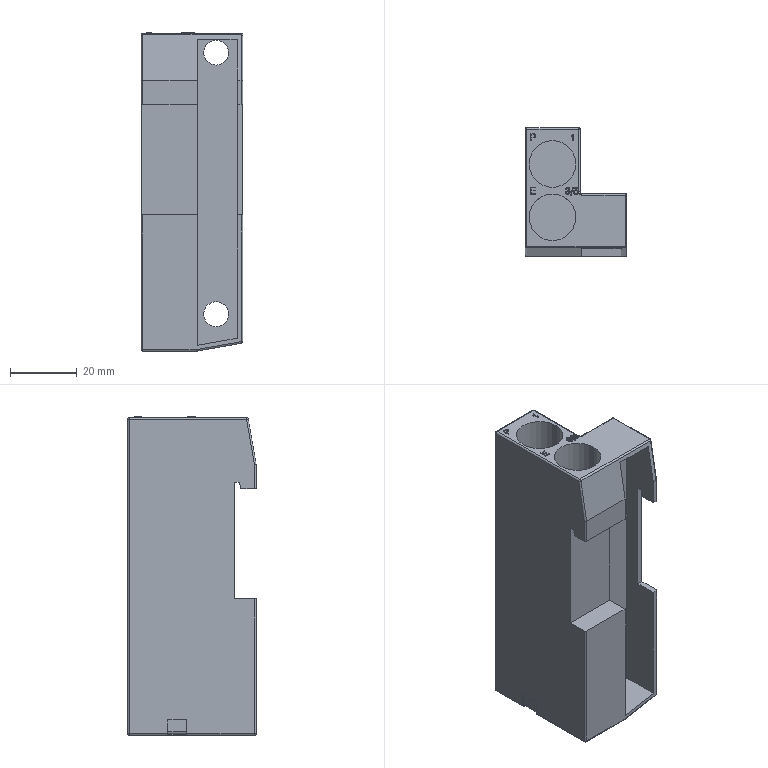Part | STEP file | SS5V1-16S3AD-08B-N1_CAD Side End Plate | 1 solid | 174 faces | box 30.5 x 38.5 x 95.55 mm | volume 62940 mm3 | plane 91 | cylinder 39 | spline 30 | sphere 12 | torus 2 | commonest cylinder face diameters 1 x25 2.5 x4 7.5 x4 14 x4 0.5 x1 1.5 x1